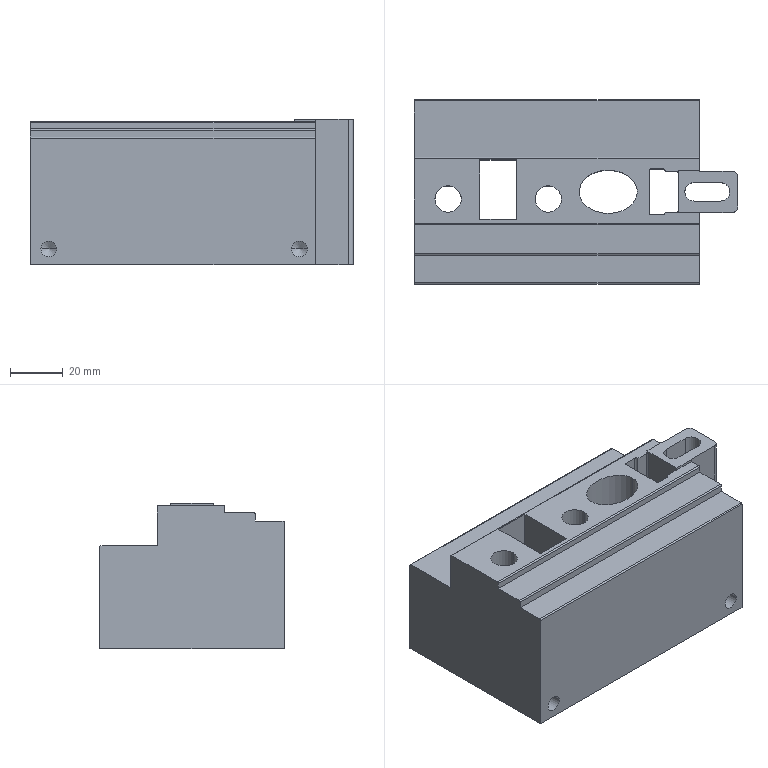Part | STEP file | KHUON DUONG | 1 solid | 91 faces | box 122.5 x 70 x 55.2 mm | volume 288291 mm3 | plane 37 | cylinder 36 | cone 16 | spline 2 | commonest cylinder face diameters 6 x8 18 x8 1 x7 1.6 x4 10 x4 7 x3